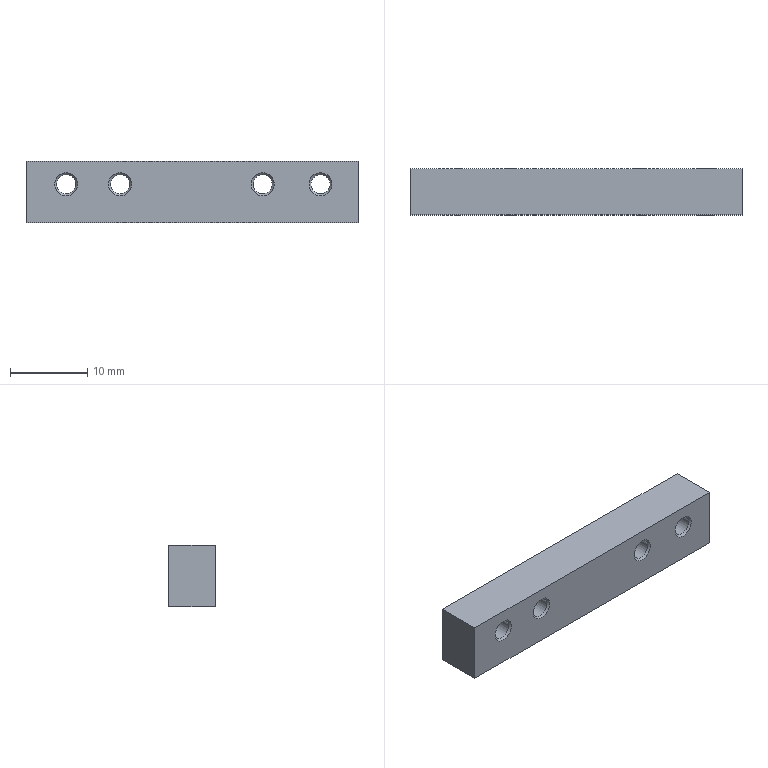Part | STEP file | VSWR protection spacer strip | 1 solid | 24 faces | box 43.08 x 5.97 x 8 mm | volume 1913 mm3 | cone 12 | plane 6 | cylinder 6 | commonest cylinder face diameters 2.5 x4 1.6 x2